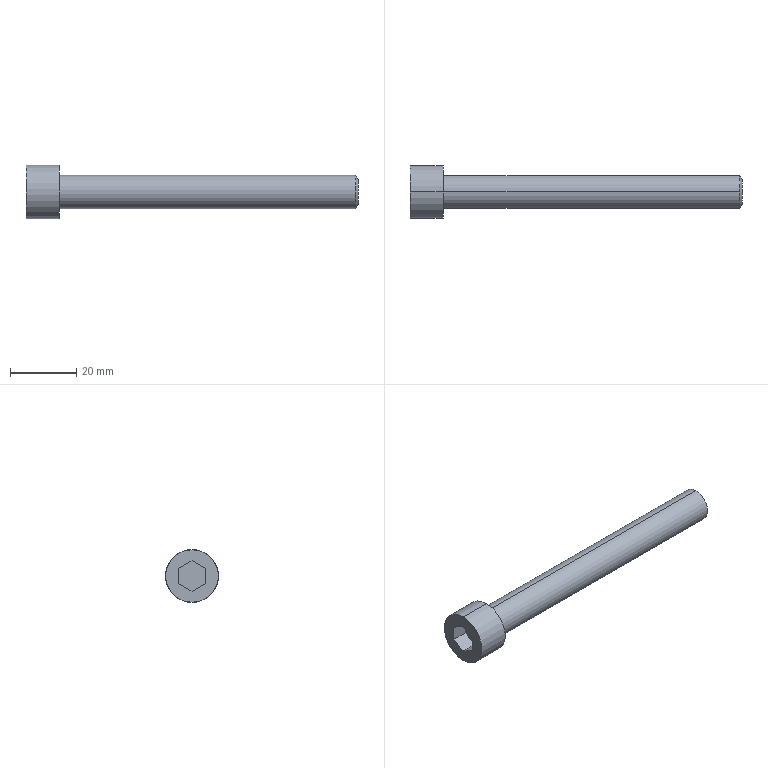Part | SolidWorks | features BlendCut 1, Cut 1, Fillet 1, LPattern 1, RevCut 1, Revolution 1 | 1 solid | 20 faces | box 100 x 16 x 16 mm | volume 8793 mm3 | plane 10 | torus 4 | cylinder 4 | cone 2 | commonest cylinder face diameters 10 x2 16 x2
STEP:
#1=CARTESIAN_POINT('',(0.,0.,7.9));
#2=VERTEX_POINT('',#1);
#3=CARTESIAN_POINT('',(0.,0.,-7.9));
#4=VERTEX_POINT('',#3);
#5=CARTESIAN_POINT('',(0.,0.,0.));
#6=DIRECTION('',(-1.,0.,0.));
#7=DIRECTION('',(0.,0.,-1.));
#8=AXIS2_PLACEMENT_3D('',#5,#6,#7);
#9=CIRCLE('',#8,7.9);
#10=EDGE_CURVE('',#2,#4,#9,.T.);
#11=ORIENTED_EDGE('',*,*,#10,.F.);
#12=CARTESIAN_POINT('',(0.1,0.,8.));
#13=VERTEX_POINT('',#12);
#14=CARTESIAN_POINT('',(0.1,0.,7.9));
#15=DIRECTION('',(0.,1.,0.));
#16=DIRECTION('',(0.,0.,1.));
#17=AXIS2_PLACEMENT_3D('',#14,#15,#16);
#18=CIRCLE('',#17,0.1);
#19=EDGE_CURVE('',#2,#13,#18,.T.);
#20=ORIENTED_EDGE('',*,*,#19,.T.);
#21=CARTESIAN_POINT('',(0.1,0.,-8.));
#22=VERTEX_POINT('',#21);
#23=CARTESIAN_POINT('',(0.1,0.,0.));
#24=DIRECTION('',(1.,0.,0.));
#25=DIRECTION('',(0.,0.,-1.));
#26=AXIS2_PLACEMENT_3D('',#23,#24,#25);
#27=CIRCLE('',#26,8.);
#28=EDGE_CURVE('',#22,#13,#27,.T.);
#29=ORIENTED_EDGE('',*,*,#28,.F.);
#30=CARTESIAN_POINT('',(0.1,0.,-7.9));
#31=DIRECTION('',(0.,-1.,0.));
#32=DIRECTION('',(0.,0.,-1.));
#33=AXIS2_PLACEMENT_3D('',#30,#31,#32);
#34=CIRCLE('',#33,0.1);
#35=EDGE_CURVE('',#4,#22,#34,.T.);
#36=ORIENTED_EDGE('',*,*,#35,.F.);
#37=EDGE_LOOP('',(#11,#20,#29,#36));
#38=FACE_OUTER_BOUND('',#37,.T.);
#39=CARTESIAN_POINT('',(0.1,0.,0.));
#40=DIRECTION('',(1.,0.,0.));
#41=DIRECTION('',(0.,0.,-1.));
#42=AXIS2_PLACEMENT_3D('',#39,#40,#41);
#43=TOROIDAL_SURFACE('',#42,7.9,0.1);
#44=ADVANCED_FACE('',(#38),#43,.T.);
#45=CARTESIAN_POINT('',(100.,0.,3.701));
#46=VERTEX_POINT('',#45);
#47=CARTESIAN_POINT('',(100.,0.,-3.701));
#48=VERTEX_POINT('',#47);
#49=CARTESIAN_POINT('',(100.,0.,0.));
#50=DIRECTION('',(-1.,0.,0.));
#51=DIRECTION('',(0.,0.,1.));
#52=AXIS2_PLACEMENT_3D('',#49,#50,#51);
#53=CIRCLE('',#52,3.701);
#54=EDGE_CURVE('',#46,#48,#53,.T.);
#55=ORIENTED_EDGE('',*,*,#54,.T.);
#56=CARTESIAN_POINT('',(99.25,0.,-5.));
#57=VERTEX_POINT('',#56);
#58=CARTESIAN_POINT('',(99.25,0.,-5.));
#59=DIRECTION('',(-0.5,0.,-0.866));
#60=VECTOR('',#59,1000.);
#61=LINE('',#58,#60);
#62=EDGE_CURVE('',#48,#57,#61,.T.);
#63=ORIENTED_EDGE('',*,*,#62,.T.);
#64=CARTESIAN_POINT('',(99.25,0.,5.));
#65=VERTEX_POINT('',#64);
#66=CARTESIAN_POINT('',(99.25,0.,0.));
#67=DIRECTION('',(-1.,0.,0.));
#68=DIRECTION('',(0.,0.,1.));
#69=AXIS2_PLACEMENT_3D('',#66,#67,#68);
#70=CIRCLE('',#69,5.);
#71=EDGE_CURVE('',#65,#57,#70,.T.);
#72=ORIENTED_EDGE('',*,*,#71,.F.);
#73=CARTESIAN_POINT('',(99.25,0.,5.));
#74=DIRECTION('',(-0.5,0.,0.866));
#75=VECTOR('',#74,1000.);
#76=LINE('',#73,#75);
#77=EDGE_CURVE('',#46,#65,#76,.T.);
#78=ORIENTED_EDGE('',*,*,#77,.F.);
#79=EDGE_LOOP('',(#55,#63,#72,#78));
#80=FACE_OUTER_BOUND('',#79,.T.);
#81=CARTESIAN_POINT('',(99.25,0.,0.));
#82=DIRECTION('',(-1.,0.,0.));
#83=DIRECTION('',(0.,0.,1.));
#84=AXIS2_PLACEMENT_3D('',#81,#82,#83);
#85=CONICAL_SURFACE('',#84,5.,1.047);
#86=ADVANCED_FACE('',(#80),#85,.T.);
#87=CARTESIAN_POINT('',(10.,0.,-5.2));
#88=VERTEX_POINT('',#87);
#89=CARTESIAN_POINT('',(10.,0.,5.2));
#90=VERTEX_POINT('',#89);
#91=CARTESIAN_POINT('',(10.,0.,0.));
#92=DIRECTION('',(-1.,0.,0.));
#93=DIRECTION('',(0.,0.,1.));
#94=AXIS2_PLACEMENT_3D('',#91,#92,#93);
#95=CIRCLE('',#94,5.2);
#96=EDGE_CURVE('',#88,#90,#95,.T.);
#97=ORIENTED_EDGE('',*,*,#96,.F.);
#98=CARTESIAN_POINT('',(10.2,0.,-5.));
#99=VERTEX_POINT('',#98);
#100=CARTESIAN_POINT('',(10.2,0.,-5.2));
#101=DIRECTION('',(0.,1.,0.));
#102=DIRECTION('',(0.,0.,1.));
#103=AXIS2_PLACEMENT_3D('',#100,#101,#102);
#104=CIRCLE('',#103,0.2);
#105=EDGE_CURVE('',#88,#99,#104,.T.);
#106=ORIENTED_EDGE('',*,*,#105,.T.);
#107=CARTESIAN_POINT('',(10.2,0.,5.));
#108=VERTEX_POINT('',#107);
#109=CARTESIAN_POINT('',(10.2,0.,0.));
#110=DIRECTION('',(-1.,0.,0.));
#111=DIRECTION('',(0.,0.,1.));
#112=AXIS2_PLACEMENT_3D('',#109,#110,#111);
#113=CIRCLE('',#112,5.);
#114=EDGE_CURVE('',#99,#108,#113,.T.);
#115=ORIENTED_EDGE('',*,*,#114,.T.);
#116=CARTESIAN_POINT('',(10.2,0.,5.2));
#117=DIRECTION('',(0.,-1.,0.));
#118=DIRECTION('',(0.,0.,-1.));
#119=AXIS2_PLACEMENT_3D('',#116,#117,#118);
#120=CIRCLE('',#119,0.2);
#121=EDGE_CURVE('',#90,#108,#120,.T.);
#122=ORIENTED_EDGE('',*,*,#121,.F.);
#123=EDGE_LOOP('',(#97,#106,#115,#122));
#124=FACE_OUTER_BOUND('',#123,.T.);
#125=CARTESIAN_POINT('',(10.2,0.,0.));
#126=DIRECTION('',(-1.,0.,0.));
#127=DIRECTION('',(0.,0.,1.));
#128=AXIS2_PLACEMENT_3D('',#125,#126,#127);
#129=TOROIDAL_SURFACE('',#128,5.2,0.2);
#130=ADVANCED_FACE('',(#124),#129,.F.);
#131=CARTESIAN_POINT('',(10.,0.,8.));
#132=VERTEX_POINT('',#131);
#133=CARTESIAN_POINT('',(10.,0.,-8.));
#134=VERTEX_POINT('',#133);
#135=CARTESIAN_POINT('',(10.,0.,0.));
#136=DIRECTION('',(-1.,0.,0.));
#137=DIRECTION('',(0.,0.,1.));
#138=AXIS2_PLACEMENT_3D('',#135,#136,#137);
#139=CIRCLE('',#138,8.);
#140=EDGE_CURVE('',#132,#134,#139,.T.);
#141=ORIENTED_EDGE('',*,*,#140,.T.);
#142=CARTESIAN_POINT('',(0.,0.,-8.));
#143=DIRECTION('',(-1.,0.,0.));
#144=VECTOR('',#143,1000.);
#145=LINE('',#142,#144);
#146=EDGE_CURVE('',#134,#22,#145,.T.);
#147=ORIENTED_EDGE('',*,*,#146,.T.);
#148=ORIENTED_EDGE('',*,*,#28,.T.);
#149=CARTESIAN_POINT('',(0.,0.,8.));
#150=DIRECTION('',(-1.,0.,0.));
#151=VECTOR('',#150,1000.);
#152=LINE('',#149,#151);
#153=EDGE_CURVE('',#132,#13,#152,.T.);
#154=ORIENTED_EDGE('',*,*,#153,.F.);
#155=EDGE_LOOP('',(#141,#147,#148,#154));
#156=FACE_OUTER_BOUND('',#155,.T.);
#157=CARTESIAN_POINT('',(0.,0.,0.));
#158=DIRECTION('',(-1.,0.,0.));
#159=DIRECTION('',(0.,0.,1.));
#160=AXIS2_PLACEMENT_3D('',#157,#158,#159);
#161=CYLINDRICAL_SURFACE('',#160,8.);
#162=ADVANCED_FACE('',(#156),#161,.T.);
#163=ORIENTED_EDGE('',*,*,#71,.T.);
#164=CARTESIAN_POINT('',(0.,0.,-5.));
#165=DIRECTION('',(-1.,0.,0.));
#166=VECTOR('',#165,1000.);
#167=LINE('',#164,#166);
#168=EDGE_CURVE('',#57,#99,#167,.T.);
#169=ORIENTED_EDGE('',*,*,#168,.T.);
#170=CARTESIAN_POINT('',(10.2,0.,0.));
#171=DIRECTION('',(-1.,0.,0.));
#172=DIRECTION('',(0.,0.,1.));
#173=AXIS2_PLACEMENT_3D('',#170,#171,#172);
#174=CIRCLE('',#173,5.);
#175=EDGE_CURVE('',#108,#99,#174,.T.);
#176=ORIENTED_EDGE('',*,*,#175,.F.);
#177=CARTESIAN_POINT('',(0.,0.,5.));
#178=DIRECTION('',(-1.,0.,0.));
#179=VECTOR('',#178,1000.);
#180=LINE('',#177,#179);
#181=EDGE_CURVE('',#65,#108,#180,.T.);
#182=ORIENTED_EDGE('',*,*,#181,.F.);
#183=EDGE_LOOP('',(#163,#169,#176,#182));
#184=FACE_OUTER_BOUND('',#183,.T.);
#185=CARTESIAN_POINT('',(0.,0.,0.));
#186=DIRECTION('',(-1.,0.,0.));
#187=DIRECTION('',(0.,0.,1.));
#188=AXIS2_PLACEMENT_3D('',#185,#186,#187);
#189=CYLINDRICAL_SURFACE('',#188,5.);
#190=ADVANCED_FACE('',(#184),#189,.T.);
#191=ORIENTED_EDGE('',*,*,#168,.F.);
#192=CARTESIAN_POINT('',(99.25,0.,0.));
#193=DIRECTION('',(-1.,0.,0.));
#194=DIRECTION('',(0.,0.,1.));
#195=AXIS2_PLACEMENT_3D('',#192,#193,#194);
#196=CIRCLE('',#195,5.);
#197=EDGE_CURVE('',#57,#65,#196,.T.);
#198=ORIENTED_EDGE('',*,*,#197,.T.);
#199=ORIENTED_EDGE('',*,*,#181,.T.);
#200=ORIENTED_EDGE('',*,*,#114,.F.);
#201=EDGE_LOOP('',(#191,#198,#199,#200));
#202=FACE_OUTER_BOUND('',#201,.T.);
#203=CARTESIAN_POINT('',(0.,0.,0.));
#204=DIRECTION('',(-1.,0.,0.));
#205=DIRECTION('',(0.,0.,1.));
#206=AXIS2_PLACEMENT_3D('',#203,#204,#205);
#207=CYLINDRICAL_SURFACE('',#206,5.);
#208=ADVANCED_FACE('',(#202),#207,.T.);
#209=CARTESIAN_POINT('',(0.,0.,0.));
#210=DIRECTION('',(-1.,0.,0.));
#211=DIRECTION('',(0.,0.,-1.));
#212=AXIS2_PLACEMENT_3D('',#209,#210,#211);
#213=CIRCLE('',#212,7.9);
#214=EDGE_CURVE('',#4,#2,#213,.T.);
#215=ORIENTED_EDGE('',*,*,#214,.T.);
#216=ORIENTED_EDGE('',*,*,#10,.T.);
#217=EDGE_LOOP('',(#215,#216));
#218=FACE_OUTER_BOUND('',#217,.T.);
#219=CARTESIAN_POINT('',(0.,0.,4.575));
#220=VERTEX_POINT('',#219);
#221=CARTESIAN_POINT('',(0.,3.962,2.287));
#222=VERTEX_POINT('',#221);
#223=CARTESIAN_POINT('',(0.,0.,4.575));
#224=DIRECTION('',(0.,0.866,-0.5));
#225=VECTOR('',#224,1000.);
#226=LINE('',#223,#225);
#227=EDGE_CURVE('',#220,#222,#226,.T.);
#228=ORIENTED_EDGE('',*,*,#227,.F.);
#229=CARTESIAN_POINT('',(0.,-3.962,2.288));
#230=VERTEX_POINT('',#229);
#231=CARTESIAN_POINT('',(0.,-3.962,2.288));
#232=DIRECTION('',(0.,0.866,0.5));
#233=VECTOR('',#232,1000.);
#234=LINE('',#231,#233);
#235=EDGE_CURVE('',#230,#220,#234,.T.);
#236=ORIENTED_EDGE('',*,*,#235,.F.);
#237=CARTESIAN_POINT('',(0.,-3.962,-2.288));
#238=VERTEX_POINT('',#237);
#239=CARTESIAN_POINT('',(0.,-3.962,-2.288));
#240=DIRECTION('',(0.,0.,1.));
#241=VECTOR('',#240,1000.);
#242=LINE('',#239,#241);
#243=EDGE_CURVE('',#238,#230,#242,.T.);
#244=ORIENTED_EDGE('',*,*,#243,.F.);
#245=CARTESIAN_POINT('',(0.,0.,-4.575));
#246=VERTEX_POINT('',#245);
#247=CARTESIAN_POINT('',(0.,0.,-4.575));
#248=DIRECTION('',(0.,-0.866,0.5));
#249=VECTOR('',#248,1000.);
#250=LINE('',#247,#249);
#251=EDGE_CURVE('',#246,#238,#250,.T.);
#252=ORIENTED_EDGE('',*,*,#251,.F.);
#253=CARTESIAN_POINT('',(0.,3.962,-2.287));
#254=VERTEX_POINT('',#253);
#255=CARTESIAN_POINT('',(0.,3.962,-2.287));
#256=DIRECTION('',(0.,-0.866,-0.5));
#257=VECTOR('',#256,1000.);
#258=LINE('',#255,#257);
#259=EDGE_CURVE('',#254,#246,#258,.T.);
#260=ORIENTED_EDGE('',*,*,#259,.F.);
#261=CARTESIAN_POINT('',(0.,3.962,2.287));
#262=DIRECTION('',(0.,0.,-1.));
#263=VECTOR('',#262,1000.);
#264=LINE('',#261,#263);
#265=EDGE_CURVE('',#222,#254,#264,.T.);
#266=ORIENTED_EDGE('',*,*,#265,.F.);
#267=EDGE_LOOP('',(#228,#236,#244,#252,#260,#266));
#268=FACE_BOUND('',#267,.T.);
#269=CARTESIAN_POINT('',(0.,0.,0.));
#270=DIRECTION('',(1.,0.,0.));
#271=DIRECTION('',(0.,0.,-1.));
#272=AXIS2_PLACEMENT_3D('',#269,#270,#271);
#273=PLANE('',#272);
#274=ADVANCED_FACE('',(#218,#268),#273,.F.);
#275=ORIENTED_EDGE('',*,*,#146,.F.);
#276=CARTESIAN_POINT('',(10.,0.,0.));
#277=DIRECTION('',(-1.,0.,0.));
#278=DIRECTION('',(0.,0.,1.));
#279=AXIS2_PLACEMENT_3D('',#276,#277,#278);
#280=CIRCLE('',#279,8.);
#281=EDGE_CURVE('',#134,#132,#280,.T.);
#282=ORIENTED_EDGE('',*,*,#281,.T.);
#283=ORIENTED_EDGE('',*,*,#153,.T.);
#284=CARTESIAN_POINT('',(0.1,0.,0.));
#285=DIRECTION('',(1.,0.,0.));
#286=DIRECTION('',(0.,0.,-1.));
#287=AXIS2_PLACEMENT_3D('',#284,#285,#286);
#288=CIRCLE('',#287,8.);
#289=EDGE_CURVE('',#13,#22,#288,.T.);
#290=ORIENTED_EDGE('',*,*,#289,.T.);
#291=EDGE_LOOP('',(#275,#282,#283,#290));
#292=FACE_OUTER_BOUND('',#291,.T.);
#293=CARTESIAN_POINT('',(0.,0.,0.));
#294=DIRECTION('',(-1.,0.,0.));
#295=DIRECTION('',(0.,0.,1.));
#296=AXIS2_PLACEMENT_3D('',#293,#294,#295);
#297=CYLINDRICAL_SURFACE('',#296,8.);
#298=ADVANCED_FACE('',(#292),#297,.T.);
#299=ORIENTED_EDGE('',*,*,#140,.F.);
#300=ORIENTED_EDGE('',*,*,#281,.F.);
#301=EDGE_LOOP('',(#299,#300));
#302=FACE_OUTER_BOUND('',#301,.T.);
#303=CARTESIAN_POINT('',(10.,0.,0.));
#304=DIRECTION('',(-1.,0.,0.));
#305=DIRECTION('',(0.,0.,1.));
#306=AXIS2_PLACEMENT_3D('',#303,#304,#305);
#307=CIRCLE('',#306,5.2);
#308=EDGE_CURVE('',#90,#88,#307,.T.);
#309=ORIENTED_EDGE('',*,*,#308,.T.);
#310=ORIENTED_EDGE('',*,*,#96,.T.);
#311=EDGE_LOOP('',(#309,#310));
#312=FACE_BOUND('',#311,.T.);
#313=CARTESIAN_POINT('',(10.,8.,0.));
#314=DIRECTION('',(-1.,0.,0.));
#315=DIRECTION('',(0.,0.,1.));
#316=AXIS2_PLACEMENT_3D('',#313,#314,#315);
#317=PLANE('',#316);
#318=ADVANCED_FACE('',(#302,#312),#317,.F.);
#319=ORIENTED_EDGE('',*,*,#105,.F.);
#320=ORIENTED_EDGE('',*,*,#308,.F.);
#321=ORIENTED_EDGE('',*,*,#121,.T.);
#322=ORIENTED_EDGE('',*,*,#175,.T.);
#323=EDGE_LOOP('',(#319,#320,#321,#322));
#324=FACE_OUTER_BOUND('',#323,.T.);
#325=CARTESIAN_POINT('',(10.2,0.,0.));
#326=DIRECTION('',(-1.,0.,0.));
#327=DIRECTION('',(0.,0.,1.));
#328=AXIS2_PLACEMENT_3D('',#325,#326,#327);
#329=TOROIDAL_SURFACE('',#328,5.2,0.2);
#330=ADVANCED_FACE('',(#324),#329,.F.);
#331=ORIENTED_EDGE('',*,*,#235,.T.);
#332=CARTESIAN_POINT('',(5.,0.,4.575));
#333=VERTEX_POINT('',#332);
#334=CARTESIAN_POINT('',(5.,0.,4.575));
#335=DIRECTION('',(-1.,0.,0.));
#336=VECTOR('',#335,1000.);
#337=LINE('',#334,#336);
#338=EDGE_CURVE('',#333,#220,#337,.T.);
#339=ORIENTED_EDGE('',*,*,#338,.F.);
#340=CARTESIAN_POINT('',(5.,-3.962,2.288));
#341=VERTEX_POINT('',#340);
#342=CARTESIAN_POINT('',(5.,-3.962,2.288));
#343=DIRECTION('',(0.,0.866,0.5));
#344=VECTOR('',#343,1000.);
#345=LINE('',#342,#344);
#346=EDGE_CURVE('',#341,#333,#345,.T.);
#347=ORIENTED_EDGE('',*,*,#346,.F.);
#348=CARTESIAN_POINT('',(5.,-3.962,2.288));
#349=DIRECTION('',(-1.,0.,0.));
#350=VECTOR('',#349,1000.);
#351=LINE('',#348,#350);
#352=EDGE_CURVE('',#341,#230,#351,.T.);
#353=ORIENTED_EDGE('',*,*,#352,.T.);
#354=EDGE_LOOP('',(#331,#339,#347,#353));
#355=FACE_OUTER_BOUND('',#354,.T.);
#356=CARTESIAN_POINT('',(5.,-3.962,2.288));
#357=DIRECTION('',(0.,-0.5,0.866));
#358=DIRECTION('',(0.,-0.866,-0.5));
#359=AXIS2_PLACEMENT_3D('',#356,#357,#358);
#360=PLANE('',#359);
#361=ADVANCED_FACE('',(#355),#360,.F.);
#362=ORIENTED_EDGE('',*,*,#243,.T.);
#363=ORIENTED_EDGE('',*,*,#352,.F.);
#364=CARTESIAN_POINT('',(5.,-3.962,-2.288));
#365=VERTEX_POINT('',#364);
#366=CARTESIAN_POINT('',(5.,-3.962,-2.288));
#367=DIRECTION('',(0.,0.,1.));
#368=VECTOR('',#367,1000.);
#369=LINE('',#366,#368);
#370=EDGE_CURVE('',#365,#341,#369,.T.);
#371=ORIENTED_EDGE('',*,*,#370,.F.);
#372=CARTESIAN_POINT('',(5.,-3.962,-2.288));
#373=DIRECTION('',(-1.,0.,0.));
#374=VECTOR('',#373,1000.);
#375=LINE('',#372,#374);
#376=EDGE_CURVE('',#365,#238,#375,.T.);
#377=ORIENTED_EDGE('',*,*,#376,.T.);
#378=EDGE_LOOP('',(#362,#363,#371,#377));
#379=FACE_OUTER_BOUND('',#378,.T.);
#380=CARTESIAN_POINT('',(5.,-3.962,-2.288));
#381=DIRECTION('',(0.,-1.,0.));
#382=DIRECTION('',(0.,0.,-1.));
#383=AXIS2_PLACEMENT_3D('',#380,#381,#382);
#384=PLANE('',#383);
#385=ADVANCED_FACE('',(#379),#384,.F.);
#386=ORIENTED_EDGE('',*,*,#251,.T.);
#387=ORIENTED_EDGE('',*,*,#376,.F.);
#388=CARTESIAN_POINT('',(5.,0.,-4.575));
#389=VERTEX_POINT('',#388);
#390=CARTESIAN_POINT('',(5.,0.,-4.575));
#391=DIRECTION('',(0.,-0.866,0.5));
#392=VECTOR('',#391,1000.);
#393=LINE('',#390,#392);
#394=EDGE_CURVE('',#389,#365,#393,.T.);
#395=ORIENTED_EDGE('',*,*,#394,.F.);
#396=CARTESIAN_POINT('',(5.,0.,-4.575));
#397=DIRECTION('',(-1.,0.,0.));
#398=VECTOR('',#397,1000.);
#399=LINE('',#396,#398);
#400=EDGE_CURVE('',#389,#246,#399,.T.);
#401=ORIENTED_EDGE('',*,*,#400,.T.);
#402=EDGE_LOOP('',(#386,#387,#395,#401));
#403=FACE_OUTER_BOUND('',#402,.T.);
#404=CARTESIAN_POINT('',(5.,0.,-4.575));
#405=DIRECTION('',(0.,-0.5,-0.866));
#406=DIRECTION('',(0.,0.866,-0.5));
#407=AXIS2_PLACEMENT_3D('',#404,#405,#406);
#408=PLANE('',#407);
#409=ADVANCED_FACE('',(#403),#408,.F.);
#410=ORIENTED_EDGE('',*,*,#259,.T.);
#411=ORIENTED_EDGE('',*,*,#400,.F.);
#412=CARTESIAN_POINT('',(5.,3.962,-2.287));
#413=VERTEX_POINT('',#412);
#414=CARTESIAN_POINT('',(5.,3.962,-2.287));
#415=DIRECTION('',(0.,-0.866,-0.5));
#416=VECTOR('',#415,1000.);
#417=LINE('',#414,#416);
#418=EDGE_CURVE('',#413,#389,#417,.T.);
#419=ORIENTED_EDGE('',*,*,#418,.F.);
#420=CARTESIAN_POINT('',(5.,3.962,-2.287));
#421=DIRECTION('',(-1.,0.,0.));
#422=VECTOR('',#421,1000.);
#423=LINE('',#420,#422);
#424=EDGE_CURVE('',#413,#254,#423,.T.);
#425=ORIENTED_EDGE('',*,*,#424,.T.);
#426=EDGE_LOOP('',(#410,#411,#419,#425));
#427=FACE_OUTER_BOUND('',#426,.T.);
#428=CARTESIAN_POINT('',(5.,3.962,-2.287));
#429=DIRECTION('',(0.,0.5,-0.866));
#430=DIRECTION('',(0.,0.866,0.5));
#431=AXIS2_PLACEMENT_3D('',#428,#429,#430);
#432=PLANE('',#431);
#433=ADVANCED_FACE('',(#427),#432,.F.);
#434=ORIENTED_EDGE('',*,*,#265,.T.);
#435=ORIENTED_EDGE('',*,*,#424,.F.);
#436=CARTESIAN_POINT('',(5.,3.962,2.287));
#437=VERTEX_POINT('',#436);
#438=CARTESIAN_POINT('',(5.,3.962,2.287));
#439=DIRECTION('',(0.,0.,-1.));
#440=VECTOR('',#439,1000.);
#441=LINE('',#438,#440);
#442=EDGE_CURVE('',#437,#413,#441,.T.);
#443=ORIENTED_EDGE('',*,*,#442,.F.);
#444=CARTESIAN_POINT('',(5.,3.962,2.287));
#445=DIRECTION('',(-1.,0.,0.));
#446=VECTOR('',#445,1000.);
#447=LINE('',#444,#446);
#448=EDGE_CURVE('',#437,#222,#447,.T.);
#449=ORIENTED_EDGE('',*,*,#448,.T.);
#450=EDGE_LOOP('',(#434,#435,#443,#449));
#451=FACE_OUTER_BOUND('',#450,.T.);
#452=CARTESIAN_POINT('',(5.,3.962,2.287));
#453=DIRECTION('',(0.,1.,0.));
#454=DIRECTION('',(0.,0.,1.));
#455=AXIS2_PLACEMENT_3D('',#452,#453,#454);
#456=PLANE('',#455);
#457=ADVANCED_FACE('',(#451),#456,.F.);
#458=ORIENTED_EDGE('',*,*,#227,.T.);
#459=ORIENTED_EDGE('',*,*,#448,.F.);
#460=CARTESIAN_POINT('',(5.,0.,4.575));
#461=DIRECTION('',(0.,0.866,-0.5));
#462=VECTOR('',#461,1000.);
#463=LINE('',#460,#462);
#464=EDGE_CURVE('',#333,#437,#463,.T.);
#465=ORIENTED_EDGE('',*,*,#464,.F.);
#466=ORIENTED_EDGE('',*,*,#338,.T.);
#467=EDGE_LOOP('',(#458,#459,#465,#466));
#468=FACE_OUTER_BOUND('',#467,.T.);
#469=CARTESIAN_POINT('',(5.,0.,4.575));
#470=DIRECTION('',(0.,0.5,0.866));
#471=DIRECTION('',(0.,-0.866,0.5));
#472=AXIS2_PLACEMENT_3D('',#469,#470,#471);
#473=PLANE('',#472);
#474=ADVANCED_FACE('',(#468),#473,.F.);
#475=ORIENTED_EDGE('',*,*,#346,.T.);
#476=ORIENTED_EDGE('',*,*,#464,.T.);
#477=ORIENTED_EDGE('',*,*,#442,.T.);
#478=ORIENTED_EDGE('',*,*,#418,.T.);
#479=ORIENTED_EDGE('',*,*,#394,.T.);
#480=ORIENTED_EDGE('',*,*,#370,.T.);
#481=EDGE_LOOP('',(#475,#476,#477,#478,#479,#480));
#482=FACE_OUTER_BOUND('',#481,.T.);
#483=CARTESIAN_POINT('',(5.,-3.962,2.288));
#484=DIRECTION('',(1.,0.,0.));
#485=DIRECTION('',(0.,0.,-1.));
#486=AXIS2_PLACEMENT_3D('',#483,#484,#485);
#487=PLANE('',#486);
#488=ADVANCED_FACE('',(#482),#487,.F.);
#489=ORIENTED_EDGE('',*,*,#62,.F.);
#490=CARTESIAN_POINT('',(100.,0.,0.));
#491=DIRECTION('',(-1.,0.,0.));
#492=DIRECTION('',(0.,0.,1.));
#493=AXIS2_PLACEMENT_3D('',#490,#491,#492);
#494=CIRCLE('',#493,3.701);
#495=EDGE_CURVE('',#48,#46,#494,.T.);
#496=ORIENTED_EDGE('',*,*,#495,.T.);
#497=ORIENTED_EDGE('',*,*,#77,.T.);
#498=ORIENTED_EDGE('',*,*,#197,.F.);
#499=EDGE_LOOP('',(#489,#496,#497,#498));
#500=FACE_OUTER_BOUND('',#499,.T.);
#501=CARTESIAN_POINT('',(99.25,0.,0.));
#502=DIRECTION('',(-1.,0.,0.));
#503=DIRECTION('',(0.,0.,1.));
#504=AXIS2_PLACEMENT_3D('',#501,#502,#503);
#505=CONICAL_SURFACE('',#504,5.,1.047);
#506=ADVANCED_FACE('',(#500),#505,.T.);
#507=ORIENTED_EDGE('',*,*,#54,.F.);
#508=ORIENTED_EDGE('',*,*,#495,.F.);
#509=EDGE_LOOP('',(#507,#508));
#510=FACE_OUTER_BOUND('',#509,.T.);
#511=CARTESIAN_POINT('',(100.,5.,0.));
#512=DIRECTION('',(-1.,0.,0.));
#513=DIRECTION('',(0.,0.,1.));
#514=AXIS2_PLACEMENT_3D('',#511,#512,#513);
#515=PLANE('',#514);
#516=ADVANCED_FACE('',(#510),#515,.F.);
#517=ORIENTED_EDGE('',*,*,#19,.F.);
#518=ORIENTED_EDGE('',*,*,#214,.F.);
#519=ORIENTED_EDGE('',*,*,#35,.T.);
#520=ORIENTED_EDGE('',*,*,#289,.F.);
#521=EDGE_LOOP('',(#517,#518,#519,#520));
#522=FACE_OUTER_BOUND('',#521,.T.);
#523=CARTESIAN_POINT('',(0.1,0.,0.));
#524=DIRECTION('',(1.,0.,0.));
#525=DIRECTION('',(0.,0.,-1.));
#526=AXIS2_PLACEMENT_3D('',#523,#524,#525);
#527=TOROIDAL_SURFACE('',#526,7.9,0.1);
#528=ADVANCED_FACE('',(#522),#527,.T.);
#529=CLOSED_SHELL('',(#44,#86,#130,#162,#190,#208,#274,#298,#318,#330,#361,#385,#409,#433,#457,#474,#488,#506,#516,#528));
#530=MANIFOLD_SOLID_BREP('',#529);
#531=CARTESIAN_POINT('',(0.,0.,0.));
#532=DIRECTION('',(0.,0.,1.));
#533=DIRECTION('',(1.,0.,0.));
#534=AXIS2_PLACEMENT_3D('',#531,#532,#533);
#535=(LENGTH_UNIT()NAMED_UNIT(*)SI_UNIT(.MILLI.,.METRE.));
#536=UNCERTAINTY_MEASURE_WITH_UNIT(LENGTH_MEASURE(0.00001),#535,'','');
#537=(NAMED_UNIT(*)PLANE_ANGLE_UNIT()SI_UNIT($,.RADIAN.));
#538=(NAMED_UNIT(*)SI_UNIT($,.STERADIAN.)SOLID_ANGLE_UNIT());
#539=(GEOMETRIC_REPRESENTATION_CONTEXT(3)GLOBAL_UNCERTAINTY_ASSIGNED_CONTEXT((#536))GLOBAL_UNIT_ASSIGNED_CONTEXT((#535,#537,#538))REPRESENTATION_CONTEXT('',''));
#540=ADVANCED_BREP_SHAPE_REPRESENTATION('',(#530,#534),#539);